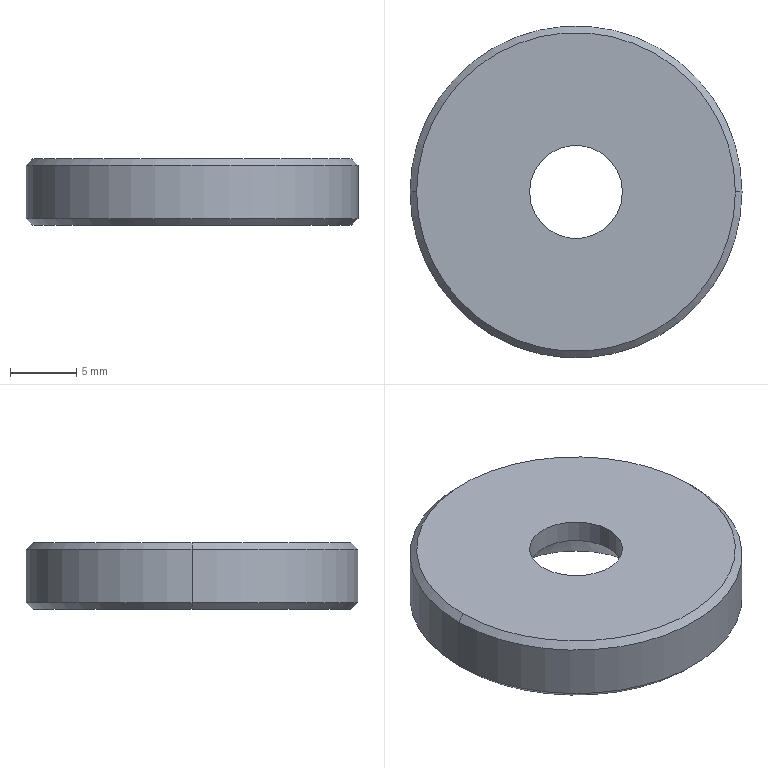Part | Creo | 1 solid | 12 faces | box 25 x 25 x 5 mm | volume 2085 mm3 | cone 6 | cylinder 4 | plane 2 | commonest cylinder face diameters 7 x2 25 x2
STEP:
#1=CARTESIAN_POINT('',(148.,-315.,-300.5));
#2=VERTEX_POINT('',#1);
#3=CARTESIAN_POINT('',(172.,-315.,-300.5));
#4=VERTEX_POINT('',#3);
#5=CARTESIAN_POINT('',(160.,-315.,-300.5));
#6=DIRECTION('',(0.,0.,-1.));
#7=DIRECTION('',(-1.,0.,0.));
#8=AXIS2_PLACEMENT_3D('',#5,#6,#7);
#9=CIRCLE('',#8,12.);
#10=EDGE_CURVE('',#2,#4,#9,.T.);
#11=ORIENTED_EDGE('',*,*,#10,.F.);
#12=CARTESIAN_POINT('',(160.,-315.,-300.5));
#13=DIRECTION('',(0.,0.,-1.));
#14=DIRECTION('',(1.,0.,0.));
#15=AXIS2_PLACEMENT_3D('',#12,#13,#14);
#16=CIRCLE('',#15,12.);
#17=EDGE_CURVE('',#4,#2,#16,.T.);
#18=ORIENTED_EDGE('',*,*,#17,.F.);
#19=EDGE_LOOP('',(#11,#18));
#20=FACE_OUTER_BOUND('',#19,.F.);
#21=CARTESIAN_POINT('',(153.2,-315.,-300.5));
#22=VERTEX_POINT('',#21);
#23=CARTESIAN_POINT('',(166.8,-315.,-300.5));
#24=VERTEX_POINT('',#23);
#25=CARTESIAN_POINT('',(160.,-315.,-300.5));
#26=DIRECTION('',(0.,0.,1.));
#27=DIRECTION('',(-1.,0.,0.));
#28=AXIS2_PLACEMENT_3D('',#25,#26,#27);
#29=CIRCLE('',#28,6.8);
#30=EDGE_CURVE('',#22,#24,#29,.T.);
#31=ORIENTED_EDGE('',*,*,#30,.F.);
#32=CARTESIAN_POINT('',(160.,-315.,-300.5));
#33=DIRECTION('',(0.,0.,1.));
#34=DIRECTION('',(1.,0.,0.));
#35=AXIS2_PLACEMENT_3D('',#32,#33,#34);
#36=CIRCLE('',#35,6.8);
#37=EDGE_CURVE('',#24,#22,#36,.T.);
#38=ORIENTED_EDGE('',*,*,#37,.F.);
#39=EDGE_LOOP('',(#31,#38));
#40=FACE_BOUND('',#39,.F.);
#41=CARTESIAN_POINT('',(160.,-315.,-300.5));
#42=DIRECTION('',(0.,0.,-1.));
#43=DIRECTION('',(-1.,0.,0.));
#44=AXIS2_PLACEMENT_3D('',#41,#42,#43);
#45=PLANE('',#44);
#46=ADVANCED_FACE('',(#20,#40),#45,.T.);
#47=CARTESIAN_POINT('',(156.5,-315.,-297.2));
#48=VERTEX_POINT('',#47);
#49=CARTESIAN_POINT('',(163.5,-315.,-297.2));
#50=VERTEX_POINT('',#49);
#51=CARTESIAN_POINT('',(160.,-315.,-297.2));
#52=DIRECTION('',(0.,0.,1.));
#53=DIRECTION('',(-1.,0.,0.));
#54=AXIS2_PLACEMENT_3D('',#51,#52,#53);
#55=CIRCLE('',#54,3.5);
#56=EDGE_CURVE('',#48,#50,#55,.T.);
#57=ORIENTED_EDGE('',*,*,#56,.F.);
#58=CARTESIAN_POINT('',(156.5,-315.,-297.2));
#59=DIRECTION('',(-0.7071,0.,-0.7071));
#60=VECTOR('',#59,4.667);
#61=LINE('',#58,#60);
#62=EDGE_CURVE('',#48,#22,#61,.T.);
#63=ORIENTED_EDGE('',*,*,#62,.T.);
#64=ORIENTED_EDGE('',*,*,#30,.T.);
#65=CARTESIAN_POINT('',(163.5,-315.,-297.2));
#66=DIRECTION('',(0.7071,0.,-0.7071));
#67=VECTOR('',#66,4.667);
#68=LINE('',#65,#67);
#69=EDGE_CURVE('',#50,#24,#68,.T.);
#70=ORIENTED_EDGE('',*,*,#69,.F.);
#71=EDGE_LOOP('',(#57,#63,#64,#70));
#72=FACE_OUTER_BOUND('',#71,.F.);
#73=CARTESIAN_POINT('',(160.,-315.,-298.85));
#74=DIRECTION('',(0.,0.,-1.));
#75=DIRECTION('',(-1.,0.,0.));
#76=AXIS2_PLACEMENT_3D('',#73,#74,#75);
#77=CONICAL_SURFACE('',#76,5.15,45.);
#78=ADVANCED_FACE('',(#72),#77,.F.);
#79=CARTESIAN_POINT('',(163.5,-315.,-295.5));
#80=VERTEX_POINT('',#79);
#81=CARTESIAN_POINT('',(156.5,-315.,-295.5));
#82=VERTEX_POINT('',#81);
#83=CARTESIAN_POINT('',(160.,-315.,-295.5));
#84=DIRECTION('',(0.,0.,-1.));
#85=DIRECTION('',(1.,0.,0.));
#86=AXIS2_PLACEMENT_3D('',#83,#84,#85);
#87=CIRCLE('',#86,3.5);
#88=EDGE_CURVE('',#80,#82,#87,.T.);
#89=ORIENTED_EDGE('',*,*,#88,.T.);
#90=CARTESIAN_POINT('',(156.5,-315.,-295.5));
#91=DIRECTION('',(0.,0.,-1.));
#92=VECTOR('',#91,1.7);
#93=LINE('',#90,#92);
#94=EDGE_CURVE('',#82,#48,#93,.T.);
#95=ORIENTED_EDGE('',*,*,#94,.T.);
#96=ORIENTED_EDGE('',*,*,#56,.T.);
#97=CARTESIAN_POINT('',(163.5,-315.,-295.5));
#98=DIRECTION('',(0.,0.,-1.));
#99=VECTOR('',#98,1.7);
#100=LINE('',#97,#99);
#101=EDGE_CURVE('',#80,#50,#100,.T.);
#102=ORIENTED_EDGE('',*,*,#101,.F.);
#103=EDGE_LOOP('',(#89,#95,#96,#102));
#104=FACE_OUTER_BOUND('',#103,.F.);
#105=CARTESIAN_POINT('',(160.,-315.,-300.307));
#106=DIRECTION('',(0.,0.,-1.));
#107=DIRECTION('',(-1.,0.,0.));
#108=AXIS2_PLACEMENT_3D('',#105,#106,#107);
#109=CYLINDRICAL_SURFACE('',#108,3.5);
#110=ADVANCED_FACE('',(#104),#109,.F.);
#111=CARTESIAN_POINT('',(172.,-315.,-295.5));
#112=VERTEX_POINT('',#111);
#113=CARTESIAN_POINT('',(148.,-315.,-295.5));
#114=VERTEX_POINT('',#113);
#115=CARTESIAN_POINT('',(160.,-315.,-295.5));
#116=DIRECTION('',(0.,0.,1.));
#117=DIRECTION('',(1.,0.,0.));
#118=AXIS2_PLACEMENT_3D('',#115,#116,#117);
#119=CIRCLE('',#118,12.);
#120=EDGE_CURVE('',#112,#114,#119,.T.);
#121=ORIENTED_EDGE('',*,*,#120,.F.);
#122=CARTESIAN_POINT('',(160.,-315.,-295.5));
#123=DIRECTION('',(0.,0.,1.));
#124=DIRECTION('',(-1.,0.,0.));
#125=AXIS2_PLACEMENT_3D('',#122,#123,#124);
#126=CIRCLE('',#125,12.);
#127=EDGE_CURVE('',#114,#112,#126,.T.);
#128=ORIENTED_EDGE('',*,*,#127,.F.);
#129=EDGE_LOOP('',(#121,#128));
#130=FACE_OUTER_BOUND('',#129,.F.);
#131=ORIENTED_EDGE('',*,*,#88,.F.);
#132=CARTESIAN_POINT('',(160.,-315.,-295.5));
#133=DIRECTION('',(0.,0.,-1.));
#134=DIRECTION('',(-1.,0.,0.));
#135=AXIS2_PLACEMENT_3D('',#132,#133,#134);
#136=CIRCLE('',#135,3.5);
#137=EDGE_CURVE('',#82,#80,#136,.T.);
#138=ORIENTED_EDGE('',*,*,#137,.F.);
#139=EDGE_LOOP('',(#131,#138));
#140=FACE_BOUND('',#139,.F.);
#141=CARTESIAN_POINT('',(160.,-315.,-295.5));
#142=DIRECTION('',(0.,0.,1.));
#143=DIRECTION('',(1.,0.,0.));
#144=AXIS2_PLACEMENT_3D('',#141,#142,#143);
#145=PLANE('',#144);
#146=ADVANCED_FACE('',(#130,#140),#145,.T.);
#147=ORIENTED_EDGE('',*,*,#137,.T.);
#148=ORIENTED_EDGE('',*,*,#101,.T.);
#149=CARTESIAN_POINT('',(160.,-315.,-297.2));
#150=DIRECTION('',(0.,0.,1.));
#151=DIRECTION('',(1.,0.,0.));
#152=AXIS2_PLACEMENT_3D('',#149,#150,#151);
#153=CIRCLE('',#152,3.5);
#154=EDGE_CURVE('',#50,#48,#153,.T.);
#155=ORIENTED_EDGE('',*,*,#154,.T.);
#156=ORIENTED_EDGE('',*,*,#94,.F.);
#157=EDGE_LOOP('',(#147,#148,#155,#156));
#158=FACE_OUTER_BOUND('',#157,.F.);
#159=CARTESIAN_POINT('',(160.,-315.,-300.307));
#160=DIRECTION('',(0.,0.,-1.));
#161=DIRECTION('',(-1.,0.,0.));
#162=AXIS2_PLACEMENT_3D('',#159,#160,#161);
#163=CYLINDRICAL_SURFACE('',#162,3.5);
#164=ADVANCED_FACE('',(#158),#163,.F.);
#165=ORIENTED_EDGE('',*,*,#154,.F.);
#166=ORIENTED_EDGE('',*,*,#69,.T.);
#167=ORIENTED_EDGE('',*,*,#37,.T.);
#168=ORIENTED_EDGE('',*,*,#62,.F.);
#169=EDGE_LOOP('',(#165,#166,#167,#168));
#170=FACE_OUTER_BOUND('',#169,.F.);
#171=CARTESIAN_POINT('',(160.,-315.,-298.85));
#172=DIRECTION('',(0.,0.,-1.));
#173=DIRECTION('',(-1.,0.,0.));
#174=AXIS2_PLACEMENT_3D('',#171,#172,#173);
#175=CONICAL_SURFACE('',#174,5.15,45.);
#176=ADVANCED_FACE('',(#170),#175,.F.);
#177=CARTESIAN_POINT('',(172.5,-315.,-296.));
#178=VERTEX_POINT('',#177);
#179=CARTESIAN_POINT('',(147.5,-315.,-296.));
#180=VERTEX_POINT('',#179);
#181=CARTESIAN_POINT('',(160.,-315.,-296.));
#182=DIRECTION('',(0.,0.,1.));
#183=DIRECTION('',(1.,0.,0.));
#184=AXIS2_PLACEMENT_3D('',#181,#182,#183);
#185=CIRCLE('',#184,12.5);
#186=EDGE_CURVE('',#178,#180,#185,.T.);
#187=ORIENTED_EDGE('',*,*,#186,.F.);
#188=CARTESIAN_POINT('',(172.,-315.,-295.5));
#189=DIRECTION('',(0.7071,0.,-0.7071));
#190=VECTOR('',#189,0.7071);
#191=LINE('',#188,#190);
#192=EDGE_CURVE('',#112,#178,#191,.T.);
#193=ORIENTED_EDGE('',*,*,#192,.F.);
#194=ORIENTED_EDGE('',*,*,#120,.T.);
#195=CARTESIAN_POINT('',(148.,-315.,-295.5));
#196=DIRECTION('',(-0.7071,0.,-0.7071));
#197=VECTOR('',#196,0.7071);
#198=LINE('',#195,#197);
#199=EDGE_CURVE('',#114,#180,#198,.T.);
#200=ORIENTED_EDGE('',*,*,#199,.T.);
#201=EDGE_LOOP('',(#187,#193,#194,#200));
#202=FACE_OUTER_BOUND('',#201,.F.);
#203=CARTESIAN_POINT('',(160.,-315.,-295.75));
#204=DIRECTION('',(0.,0.,-1.));
#205=DIRECTION('',(-1.,0.,0.));
#206=AXIS2_PLACEMENT_3D('',#203,#204,#205);
#207=CONICAL_SURFACE('',#206,12.25,45.);
#208=ADVANCED_FACE('',(#202),#207,.T.);
#209=ORIENTED_EDGE('',*,*,#186,.T.);
#210=CARTESIAN_POINT('',(147.5,-315.,-300.));
#211=VERTEX_POINT('',#210);
#212=CARTESIAN_POINT('',(147.5,-315.,-296.));
#213=DIRECTION('',(0.,0.,-1.));
#214=VECTOR('',#213,4.);
#215=LINE('',#212,#214);
#216=EDGE_CURVE('',#180,#211,#215,.T.);
#217=ORIENTED_EDGE('',*,*,#216,.T.);
#218=CARTESIAN_POINT('',(172.5,-315.,-300.));
#219=VERTEX_POINT('',#218);
#220=CARTESIAN_POINT('',(160.,-315.,-300.));
#221=DIRECTION('',(0.,0.,-1.));
#222=DIRECTION('',(-1.,0.,0.));
#223=AXIS2_PLACEMENT_3D('',#220,#221,#222);
#224=CIRCLE('',#223,12.5);
#225=EDGE_CURVE('',#211,#219,#224,.T.);
#226=ORIENTED_EDGE('',*,*,#225,.T.);
#227=CARTESIAN_POINT('',(172.5,-315.,-296.));
#228=DIRECTION('',(0.,0.,-1.));
#229=VECTOR('',#228,4.);
#230=LINE('',#227,#229);
#231=EDGE_CURVE('',#178,#219,#230,.T.);
#232=ORIENTED_EDGE('',*,*,#231,.F.);
#233=EDGE_LOOP('',(#209,#217,#226,#232));
#234=FACE_OUTER_BOUND('',#233,.F.);
#235=CARTESIAN_POINT('',(160.,-315.,-295.5));
#236=DIRECTION('',(0.,0.,-1.));
#237=DIRECTION('',(-1.,0.,0.));
#238=AXIS2_PLACEMENT_3D('',#235,#236,#237);
#239=CYLINDRICAL_SURFACE('',#238,12.5);
#240=ADVANCED_FACE('',(#234),#239,.T.);
#241=CARTESIAN_POINT('',(160.,-315.,-296.));
#242=DIRECTION('',(0.,0.,1.));
#243=DIRECTION('',(-1.,0.,0.));
#244=AXIS2_PLACEMENT_3D('',#241,#242,#243);
#245=CIRCLE('',#244,12.5);
#246=EDGE_CURVE('',#180,#178,#245,.T.);
#247=ORIENTED_EDGE('',*,*,#246,.T.);
#248=ORIENTED_EDGE('',*,*,#231,.T.);
#249=CARTESIAN_POINT('',(160.,-315.,-300.));
#250=DIRECTION('',(0.,0.,-1.));
#251=DIRECTION('',(1.,0.,0.));
#252=AXIS2_PLACEMENT_3D('',#249,#250,#251);
#253=CIRCLE('',#252,12.5);
#254=EDGE_CURVE('',#219,#211,#253,.T.);
#255=ORIENTED_EDGE('',*,*,#254,.T.);
#256=ORIENTED_EDGE('',*,*,#216,.F.);
#257=EDGE_LOOP('',(#247,#248,#255,#256));
#258=FACE_OUTER_BOUND('',#257,.F.);
#259=CARTESIAN_POINT('',(160.,-315.,-295.5));
#260=DIRECTION('',(0.,0.,-1.));
#261=DIRECTION('',(-1.,0.,0.));
#262=AXIS2_PLACEMENT_3D('',#259,#260,#261);
#263=CYLINDRICAL_SURFACE('',#262,12.5);
#264=ADVANCED_FACE('',(#258),#263,.T.);
#265=ORIENTED_EDGE('',*,*,#246,.F.);
#266=ORIENTED_EDGE('',*,*,#199,.F.);
#267=ORIENTED_EDGE('',*,*,#127,.T.);
#268=ORIENTED_EDGE('',*,*,#192,.T.);
#269=EDGE_LOOP('',(#265,#266,#267,#268));
#270=FACE_OUTER_BOUND('',#269,.F.);
#271=CARTESIAN_POINT('',(160.,-315.,-295.75));
#272=DIRECTION('',(0.,0.,-1.));
#273=DIRECTION('',(-1.,0.,0.));
#274=AXIS2_PLACEMENT_3D('',#271,#272,#273);
#275=CONICAL_SURFACE('',#274,12.25,45.);
#276=ADVANCED_FACE('',(#270),#275,.T.);
#277=ORIENTED_EDGE('',*,*,#254,.F.);
#278=CARTESIAN_POINT('',(172.,-315.,-300.5));
#279=DIRECTION('',(0.7071,0.,0.7071));
#280=VECTOR('',#279,0.7071);
#281=LINE('',#278,#280);
#282=EDGE_CURVE('',#4,#219,#281,.T.);
#283=ORIENTED_EDGE('',*,*,#282,.F.);
#284=ORIENTED_EDGE('',*,*,#17,.T.);
#285=CARTESIAN_POINT('',(148.,-315.,-300.5));
#286=DIRECTION('',(-0.7071,0.,0.7071));
#287=VECTOR('',#286,0.7071);
#288=LINE('',#285,#287);
#289=EDGE_CURVE('',#2,#211,#288,.T.);
#290=ORIENTED_EDGE('',*,*,#289,.T.);
#291=EDGE_LOOP('',(#277,#283,#284,#290));
#292=FACE_OUTER_BOUND('',#291,.F.);
#293=CARTESIAN_POINT('',(160.,-315.,-300.25));
#294=DIRECTION('',(0.,0.,1.));
#295=DIRECTION('',(1.,0.,0.));
#296=AXIS2_PLACEMENT_3D('',#293,#294,#295);
#297=CONICAL_SURFACE('',#296,12.25,45.);
#298=ADVANCED_FACE('',(#292),#297,.T.);
#299=ORIENTED_EDGE('',*,*,#225,.F.);
#300=ORIENTED_EDGE('',*,*,#289,.F.);
#301=ORIENTED_EDGE('',*,*,#10,.T.);
#302=ORIENTED_EDGE('',*,*,#282,.T.);
#303=EDGE_LOOP('',(#299,#300,#301,#302));
#304=FACE_OUTER_BOUND('',#303,.F.);
#305=CARTESIAN_POINT('',(160.,-315.,-300.25));
#306=DIRECTION('',(0.,0.,1.));
#307=DIRECTION('',(1.,0.,0.));
#308=AXIS2_PLACEMENT_3D('',#305,#306,#307);
#309=CONICAL_SURFACE('',#308,12.25,45.);
#310=ADVANCED_FACE('',(#304),#309,.T.);
#311=CLOSED_SHELL('',(#46,#78,#110,#146,#164,#176,#208,#240,#264,#276,#298,#310));
#312=MANIFOLD_SOLID_BREP('',#311);
#313=(LENGTH_UNIT()NAMED_UNIT(*)SI_UNIT(.MILLI.,.METRE.));
#314=UNCERTAINTY_MEASURE_WITH_UNIT(LENGTH_MEASURE(0.003571),#313,'','');
#315=(NAMED_UNIT(*)PLANE_ANGLE_UNIT()SI_UNIT($,.RADIAN.));
#316=PLANE_ANGLE_MEASURE_WITH_UNIT(PLANE_ANGLE_MEASURE(0.01745),#315);
#317=(CONVERSION_BASED_UNIT('DEGREE',#316)NAMED_UNIT(*)PLANE_ANGLE_UNIT());
#318=(NAMED_UNIT(*)SI_UNIT($,.STERADIAN.)SOLID_ANGLE_UNIT());
#319=(GEOMETRIC_REPRESENTATION_CONTEXT(3)GLOBAL_UNCERTAINTY_ASSIGNED_CONTEXT((#314))GLOBAL_UNIT_ASSIGNED_CONTEXT((#313,#317,#318))REPRESENTATION_CONTEXT('',''));
#320=ADVANCED_BREP_SHAPE_REPRESENTATION('',(#312),#319);